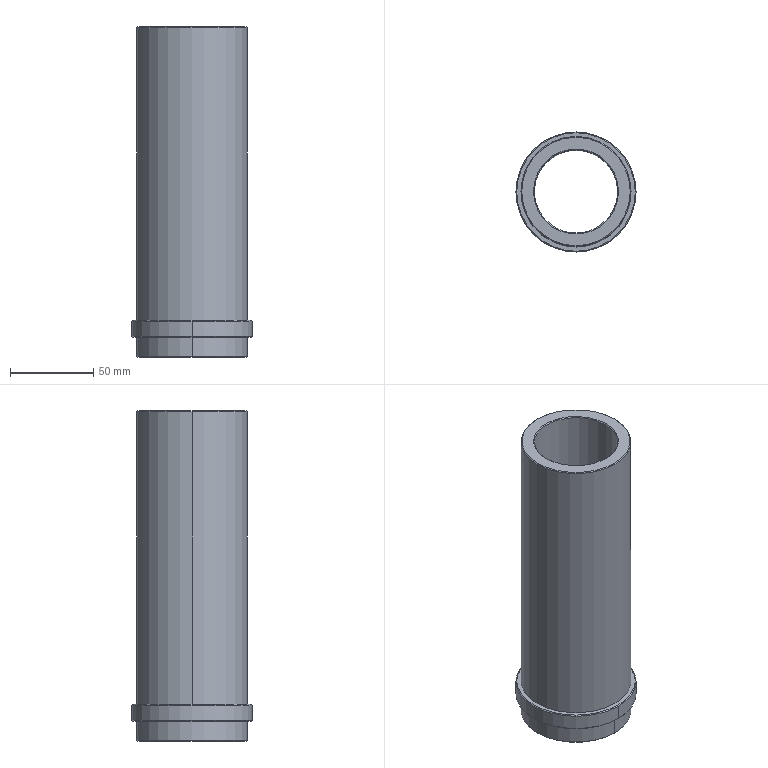Part | Creo | 1 solid | 24 faces | box 72 x 72 x 198 mm | volume 294980 mm3 | cone 12 | cylinder 8 | plane 4 | commonest cylinder face diameters 66 x4 50 x2 72 x2
STEP:
#1=CARTESIAN_POINT('',(230.,291.995,-15.5));
#2=VERTEX_POINT('',#1);
#3=CARTESIAN_POINT('',(280.,291.995,-15.5));
#4=VERTEX_POINT('',#3);
#5=CARTESIAN_POINT('',(255.,291.995,-15.5));
#6=DIRECTION('',(0.,0.,-1.));
#7=DIRECTION('',(-1.,0.,0.));
#8=AXIS2_PLACEMENT_3D('',#5,#6,#7);
#9=CIRCLE('',#8,25.);
#10=EDGE_CURVE('',#2,#4,#9,.T.);
#11=ORIENTED_EDGE('',*,*,#10,.T.);
#12=CARTESIAN_POINT('',(280.,291.995,-212.5));
#13=VERTEX_POINT('',#12);
#14=CARTESIAN_POINT('',(280.,291.995,-212.5));
#15=DIRECTION('',(0.,0.,1.));
#16=VECTOR('',#15,197.);
#17=LINE('',#14,#16);
#18=EDGE_CURVE('',#13,#4,#17,.T.);
#19=ORIENTED_EDGE('',*,*,#18,.F.);
#20=CARTESIAN_POINT('',(230.,291.995,-212.5));
#21=VERTEX_POINT('',#20);
#22=CARTESIAN_POINT('',(255.,291.995,-212.5));
#23=DIRECTION('',(0.,0.,1.));
#24=DIRECTION('',(1.,0.,0.));
#25=AXIS2_PLACEMENT_3D('',#22,#23,#24);
#26=CIRCLE('',#25,25.);
#27=EDGE_CURVE('',#13,#21,#26,.T.);
#28=ORIENTED_EDGE('',*,*,#27,.T.);
#29=CARTESIAN_POINT('',(230.,291.995,-212.5));
#30=DIRECTION('',(0.,0.,1.));
#31=VECTOR('',#30,197.);
#32=LINE('',#29,#31);
#33=EDGE_CURVE('',#21,#2,#32,.T.);
#34=ORIENTED_EDGE('',*,*,#33,.T.);
#35=EDGE_LOOP('',(#11,#19,#28,#34));
#36=FACE_OUTER_BOUND('',#35,.F.);
#37=CARTESIAN_POINT('',(255.,291.995,-201.));
#38=DIRECTION('',(0.,0.,1.));
#39=DIRECTION('',(1.,0.,0.));
#40=AXIS2_PLACEMENT_3D('',#37,#38,#39);
#41=CYLINDRICAL_SURFACE('',#40,25.);
#42=ADVANCED_FACE('',(#36),#41,.F.);
#43=CARTESIAN_POINT('',(229.5,291.995,-15.));
#44=VERTEX_POINT('',#43);
#45=CARTESIAN_POINT('',(280.5,291.995,-15.));
#46=VERTEX_POINT('',#45);
#47=CARTESIAN_POINT('',(255.,291.995,-15.));
#48=DIRECTION('',(0.,0.,-1.));
#49=DIRECTION('',(-1.,0.,0.));
#50=AXIS2_PLACEMENT_3D('',#47,#48,#49);
#51=CIRCLE('',#50,25.5);
#52=EDGE_CURVE('',#44,#46,#51,.T.);
#53=ORIENTED_EDGE('',*,*,#52,.T.);
#54=CARTESIAN_POINT('',(280.,291.995,-15.5));
#55=DIRECTION('',(0.7071,0.,0.7071));
#56=VECTOR('',#55,0.7071);
#57=LINE('',#54,#56);
#58=EDGE_CURVE('',#4,#46,#57,.T.);
#59=ORIENTED_EDGE('',*,*,#58,.F.);
#60=ORIENTED_EDGE('',*,*,#10,.F.);
#61=CARTESIAN_POINT('',(230.,291.995,-15.5));
#62=DIRECTION('',(-0.7071,0.,0.7071));
#63=VECTOR('',#62,0.7071);
#64=LINE('',#61,#63);
#65=EDGE_CURVE('',#2,#44,#64,.T.);
#66=ORIENTED_EDGE('',*,*,#65,.T.);
#67=EDGE_LOOP('',(#53,#59,#60,#66));
#68=FACE_OUTER_BOUND('',#67,.F.);
#69=CARTESIAN_POINT('',(255.,291.995,-15.25));
#70=DIRECTION('',(0.,0.,1.));
#71=DIRECTION('',(-1.,0.,0.));
#72=AXIS2_PLACEMENT_3D('',#69,#70,#71);
#73=CONICAL_SURFACE('',#72,25.25,45.);
#74=ADVANCED_FACE('',(#68),#73,.F.);
#75=CARTESIAN_POINT('',(287.5,291.995,-15.));
#76=VERTEX_POINT('',#75);
#77=CARTESIAN_POINT('',(222.5,291.995,-15.));
#78=VERTEX_POINT('',#77);
#79=CARTESIAN_POINT('',(255.,291.995,-15.));
#80=DIRECTION('',(0.,0.,1.));
#81=DIRECTION('',(1.,0.,0.));
#82=AXIS2_PLACEMENT_3D('',#79,#80,#81);
#83=CIRCLE('',#82,32.5);
#84=EDGE_CURVE('',#76,#78,#83,.T.);
#85=ORIENTED_EDGE('',*,*,#84,.F.);
#86=CARTESIAN_POINT('',(255.,291.995,-15.));
#87=DIRECTION('',(0.,0.,1.));
#88=DIRECTION('',(-1.,0.,0.));
#89=AXIS2_PLACEMENT_3D('',#86,#87,#88);
#90=CIRCLE('',#89,32.5);
#91=EDGE_CURVE('',#78,#76,#90,.T.);
#92=ORIENTED_EDGE('',*,*,#91,.F.);
#93=EDGE_LOOP('',(#85,#92));
#94=FACE_OUTER_BOUND('',#93,.F.);
#95=CARTESIAN_POINT('',(255.,291.995,-15.));
#96=DIRECTION('',(0.,0.,-1.));
#97=DIRECTION('',(1.,0.,0.));
#98=AXIS2_PLACEMENT_3D('',#95,#96,#97);
#99=CIRCLE('',#98,25.5);
#100=EDGE_CURVE('',#46,#44,#99,.T.);
#101=ORIENTED_EDGE('',*,*,#100,.F.);
#102=ORIENTED_EDGE('',*,*,#52,.F.);
#103=EDGE_LOOP('',(#101,#102));
#104=FACE_BOUND('',#103,.F.);
#105=CARTESIAN_POINT('',(-210.,43.995,-15.));
#106=DIRECTION('',(0.,0.,1.));
#107=DIRECTION('',(1.,0.,0.));
#108=AXIS2_PLACEMENT_3D('',#105,#106,#107);
#109=PLANE('',#108);
#110=ADVANCED_FACE('',(#94,#104),#109,.T.);
#111=ORIENTED_EDGE('',*,*,#100,.T.);
#112=ORIENTED_EDGE('',*,*,#65,.F.);
#113=CARTESIAN_POINT('',(255.,291.995,-15.5));
#114=DIRECTION('',(0.,0.,-1.));
#115=DIRECTION('',(1.,0.,0.));
#116=AXIS2_PLACEMENT_3D('',#113,#114,#115);
#117=CIRCLE('',#116,25.);
#118=EDGE_CURVE('',#4,#2,#117,.T.);
#119=ORIENTED_EDGE('',*,*,#118,.F.);
#120=ORIENTED_EDGE('',*,*,#58,.T.);
#121=EDGE_LOOP('',(#111,#112,#119,#120));
#122=FACE_OUTER_BOUND('',#121,.F.);
#123=CARTESIAN_POINT('',(255.,291.995,-15.25));
#124=DIRECTION('',(0.,0.,1.));
#125=DIRECTION('',(-1.,0.,0.));
#126=AXIS2_PLACEMENT_3D('',#123,#124,#125);
#127=CONICAL_SURFACE('',#126,25.25,45.);
#128=ADVANCED_FACE('',(#122),#127,.F.);
#129=ORIENTED_EDGE('',*,*,#118,.T.);
#130=ORIENTED_EDGE('',*,*,#33,.F.);
#131=CARTESIAN_POINT('',(255.,266.995,-212.5));
#132=VERTEX_POINT('',#131);
#133=CARTESIAN_POINT('',(255.,291.995,-212.5));
#134=DIRECTION('',(0.,0.,1.));
#135=DIRECTION('',(-1.,0.,0.));
#136=AXIS2_PLACEMENT_3D('',#133,#134,#135);
#137=CIRCLE('',#136,25.);
#138=EDGE_CURVE('',#21,#132,#137,.T.);
#139=ORIENTED_EDGE('',*,*,#138,.T.);
#140=CARTESIAN_POINT('',(255.,291.995,-212.5));
#141=DIRECTION('',(0.,0.,1.));
#142=DIRECTION('',(0.,-1.,0.));
#143=AXIS2_PLACEMENT_3D('',#140,#141,#142);
#144=CIRCLE('',#143,25.);
#145=EDGE_CURVE('',#132,#13,#144,.T.);
#146=ORIENTED_EDGE('',*,*,#145,.T.);
#147=ORIENTED_EDGE('',*,*,#18,.T.);
#148=EDGE_LOOP('',(#129,#130,#139,#146,#147));
#149=FACE_OUTER_BOUND('',#148,.F.);
#150=CARTESIAN_POINT('',(255.,291.995,-201.));
#151=DIRECTION('',(0.,0.,1.));
#152=DIRECTION('',(1.,0.,0.));
#153=AXIS2_PLACEMENT_3D('',#150,#151,#152);
#154=CYLINDRICAL_SURFACE('',#153,25.);
#155=ADVANCED_FACE('',(#149),#154,.F.);
#156=ORIENTED_EDGE('',*,*,#145,.F.);
#157=ORIENTED_EDGE('',*,*,#138,.F.);
#158=CARTESIAN_POINT('',(229.5,291.995,-213.));
#159=VERTEX_POINT('',#158);
#160=CARTESIAN_POINT('',(230.,291.995,-212.5));
#161=DIRECTION('',(-0.7071,0.,-0.7071));
#162=VECTOR('',#161,0.7071);
#163=LINE('',#160,#162);
#164=EDGE_CURVE('',#21,#159,#163,.T.);
#165=ORIENTED_EDGE('',*,*,#164,.T.);
#166=CARTESIAN_POINT('',(255.,266.495,-213.));
#167=VERTEX_POINT('',#166);
#168=CARTESIAN_POINT('',(255.,291.995,-213.));
#169=DIRECTION('',(0.,0.,1.));
#170=DIRECTION('',(-1.,0.,0.));
#171=AXIS2_PLACEMENT_3D('',#168,#169,#170);
#172=CIRCLE('',#171,25.5);
#173=EDGE_CURVE('',#159,#167,#172,.T.);
#174=ORIENTED_EDGE('',*,*,#173,.T.);
#175=CARTESIAN_POINT('',(280.5,291.995,-213.));
#176=VERTEX_POINT('',#175);
#177=CARTESIAN_POINT('',(255.,291.995,-213.));
#178=DIRECTION('',(0.,0.,1.));
#179=DIRECTION('',(0.,-1.,0.));
#180=AXIS2_PLACEMENT_3D('',#177,#178,#179);
#181=CIRCLE('',#180,25.5);
#182=EDGE_CURVE('',#167,#176,#181,.T.);
#183=ORIENTED_EDGE('',*,*,#182,.T.);
#184=CARTESIAN_POINT('',(280.,291.995,-212.5));
#185=DIRECTION('',(0.7071,0.,-0.7071));
#186=VECTOR('',#185,0.7071);
#187=LINE('',#184,#186);
#188=EDGE_CURVE('',#13,#176,#187,.T.);
#189=ORIENTED_EDGE('',*,*,#188,.F.);
#190=EDGE_LOOP('',(#156,#157,#165,#174,#183,#189));
#191=FACE_OUTER_BOUND('',#190,.F.);
#192=CARTESIAN_POINT('',(255.,291.995,-212.75));
#193=DIRECTION('',(0.,0.,-1.));
#194=DIRECTION('',(-1.,0.,0.));
#195=AXIS2_PLACEMENT_3D('',#192,#193,#194);
#196=CONICAL_SURFACE('',#195,25.25,45.);
#197=ADVANCED_FACE('',(#191),#196,.F.);
#198=ORIENTED_EDGE('',*,*,#27,.F.);
#199=ORIENTED_EDGE('',*,*,#188,.T.);
#200=CARTESIAN_POINT('',(255.,317.495,-213.));
#201=VERTEX_POINT('',#200);
#202=CARTESIAN_POINT('',(255.,291.995,-213.));
#203=DIRECTION('',(0.,0.,1.));
#204=DIRECTION('',(1.,0.,0.));
#205=AXIS2_PLACEMENT_3D('',#202,#203,#204);
#206=CIRCLE('',#205,25.5);
#207=EDGE_CURVE('',#176,#201,#206,.T.);
#208=ORIENTED_EDGE('',*,*,#207,.T.);
#209=CARTESIAN_POINT('',(255.,291.995,-213.));
#210=DIRECTION('',(0.,0.,1.));
#211=DIRECTION('',(0.,1.,0.));
#212=AXIS2_PLACEMENT_3D('',#209,#210,#211);
#213=CIRCLE('',#212,25.5);
#214=EDGE_CURVE('',#201,#159,#213,.T.);
#215=ORIENTED_EDGE('',*,*,#214,.T.);
#216=ORIENTED_EDGE('',*,*,#164,.F.);
#217=EDGE_LOOP('',(#198,#199,#208,#215,#216));
#218=FACE_OUTER_BOUND('',#217,.F.);
#219=CARTESIAN_POINT('',(255.,291.995,-212.75));
#220=DIRECTION('',(0.,0.,-1.));
#221=DIRECTION('',(-1.,0.,0.));
#222=AXIS2_PLACEMENT_3D('',#219,#220,#221);
#223=CONICAL_SURFACE('',#222,25.25,45.);
#224=ADVANCED_FACE('',(#218),#223,.F.);
#225=CARTESIAN_POINT('',(255.,324.495,-213.));
#226=VERTEX_POINT('',#225);
#227=CARTESIAN_POINT('',(287.5,291.995,-213.));
#228=VERTEX_POINT('',#227);
#229=CARTESIAN_POINT('',(255.,291.995,-213.));
#230=DIRECTION('',(0.,0.,-1.));
#231=DIRECTION('',(0.,1.,0.));
#232=AXIS2_PLACEMENT_3D('',#229,#230,#231);
#233=CIRCLE('',#232,32.5);
#234=EDGE_CURVE('',#226,#228,#233,.T.);
#235=ORIENTED_EDGE('',*,*,#234,.F.);
#236=CARTESIAN_POINT('',(222.5,291.995,-213.));
#237=VERTEX_POINT('',#236);
#238=CARTESIAN_POINT('',(255.,291.995,-213.));
#239=DIRECTION('',(0.,0.,-1.));
#240=DIRECTION('',(-1.,0.,0.));
#241=AXIS2_PLACEMENT_3D('',#238,#239,#240);
#242=CIRCLE('',#241,32.5);
#243=EDGE_CURVE('',#237,#226,#242,.T.);
#244=ORIENTED_EDGE('',*,*,#243,.F.);
#245=CARTESIAN_POINT('',(255.,259.495,-213.));
#246=VERTEX_POINT('',#245);
#247=CARTESIAN_POINT('',(255.,291.995,-213.));
#248=DIRECTION('',(0.,0.,-1.));
#249=DIRECTION('',(0.,-1.,0.));
#250=AXIS2_PLACEMENT_3D('',#247,#248,#249);
#251=CIRCLE('',#250,32.5);
#252=EDGE_CURVE('',#246,#237,#251,.T.);
#253=ORIENTED_EDGE('',*,*,#252,.F.);
#254=CARTESIAN_POINT('',(255.,291.995,-213.));
#255=DIRECTION('',(0.,0.,-1.));
#256=DIRECTION('',(1.,0.,0.));
#257=AXIS2_PLACEMENT_3D('',#254,#255,#256);
#258=CIRCLE('',#257,32.5);
#259=EDGE_CURVE('',#228,#246,#258,.T.);
#260=ORIENTED_EDGE('',*,*,#259,.F.);
#261=EDGE_LOOP('',(#235,#244,#253,#260));
#262=FACE_OUTER_BOUND('',#261,.F.);
#263=ORIENTED_EDGE('',*,*,#182,.F.);
#264=ORIENTED_EDGE('',*,*,#173,.F.);
#265=ORIENTED_EDGE('',*,*,#214,.F.);
#266=ORIENTED_EDGE('',*,*,#207,.F.);
#267=EDGE_LOOP('',(#263,#264,#265,#266));
#268=FACE_BOUND('',#267,.F.);
#269=CARTESIAN_POINT('',(65.,43.995,-213.));
#270=DIRECTION('',(0.,0.,-1.));
#271=DIRECTION('',(0.,1.,0.));
#272=AXIS2_PLACEMENT_3D('',#269,#270,#271);
#273=PLANE('',#272);
#274=ADVANCED_FACE('',(#262,#268),#273,.T.);
#275=CARTESIAN_POINT('',(255.,324.995,-212.5));
#276=VERTEX_POINT('',#275);
#277=CARTESIAN_POINT('',(288.,291.995,-212.5));
#278=VERTEX_POINT('',#277);
#279=CARTESIAN_POINT('',(255.,291.995,-212.5));
#280=DIRECTION('',(0.,0.,-1.));
#281=DIRECTION('',(0.,1.,0.));
#282=AXIS2_PLACEMENT_3D('',#279,#280,#281);
#283=CIRCLE('',#282,33.);
#284=EDGE_CURVE('',#276,#278,#283,.T.);
#285=ORIENTED_EDGE('',*,*,#284,.F.);
#286=CARTESIAN_POINT('',(222.,291.995,-212.5));
#287=VERTEX_POINT('',#286);
#288=CARTESIAN_POINT('',(255.,291.995,-212.5));
#289=DIRECTION('',(0.,0.,-1.));
#290=DIRECTION('',(-1.,0.,0.));
#291=AXIS2_PLACEMENT_3D('',#288,#289,#290);
#292=CIRCLE('',#291,33.);
#293=EDGE_CURVE('',#287,#276,#292,.T.);
#294=ORIENTED_EDGE('',*,*,#293,.F.);
#295=CARTESIAN_POINT('',(222.5,291.995,-213.));
#296=DIRECTION('',(-0.7071,0.,0.7071));
#297=VECTOR('',#296,0.7071);
#298=LINE('',#295,#297);
#299=EDGE_CURVE('',#237,#287,#298,.T.);
#300=ORIENTED_EDGE('',*,*,#299,.F.);
#301=ORIENTED_EDGE('',*,*,#243,.T.);
#302=ORIENTED_EDGE('',*,*,#234,.T.);
#303=CARTESIAN_POINT('',(287.5,291.995,-213.));
#304=DIRECTION('',(0.7071,0.,0.7071));
#305=VECTOR('',#304,0.7071);
#306=LINE('',#303,#305);
#307=EDGE_CURVE('',#228,#278,#306,.T.);
#308=ORIENTED_EDGE('',*,*,#307,.T.);
#309=EDGE_LOOP('',(#285,#294,#300,#301,#302,#308));
#310=FACE_OUTER_BOUND('',#309,.F.);
#311=CARTESIAN_POINT('',(255.,291.995,-212.75));
#312=DIRECTION('',(0.,0.,1.));
#313=DIRECTION('',(-1.,0.,0.));
#314=AXIS2_PLACEMENT_3D('',#311,#312,#313);
#315=CONICAL_SURFACE('',#314,32.75,45.);
#316=ADVANCED_FACE('',(#310),#315,.T.);
#317=CARTESIAN_POINT('',(255.,258.995,-212.5));
#318=VERTEX_POINT('',#317);
#319=CARTESIAN_POINT('',(255.,291.995,-212.5));
#320=DIRECTION('',(0.,0.,-1.));
#321=DIRECTION('',(1.,0.,0.));
#322=AXIS2_PLACEMENT_3D('',#319,#320,#321);
#323=CIRCLE('',#322,33.);
#324=EDGE_CURVE('',#278,#318,#323,.T.);
#325=ORIENTED_EDGE('',*,*,#324,.T.);
#326=CARTESIAN_POINT('',(255.,258.995,-201.));
#327=VERTEX_POINT('',#326);
#328=CARTESIAN_POINT('',(255.,258.995,-201.));
#329=DIRECTION('',(0.,0.,-1.));
#330=VECTOR('',#329,11.5);
#331=LINE('',#328,#330);
#332=EDGE_CURVE('',#327,#318,#331,.T.);
#333=ORIENTED_EDGE('',*,*,#332,.F.);
#334=CARTESIAN_POINT('',(255.,324.995,-201.));
#335=VERTEX_POINT('',#334);
#336=CARTESIAN_POINT('',(255.,291.995,-201.));
#337=DIRECTION('',(0.,0.,1.));
#338=DIRECTION('',(0.,-1.,0.));
#339=AXIS2_PLACEMENT_3D('',#336,#337,#338);
#340=CIRCLE('',#339,33.);
#341=EDGE_CURVE('',#327,#335,#340,.T.);
#342=ORIENTED_EDGE('',*,*,#341,.T.);
#343=CARTESIAN_POINT('',(255.,324.995,-201.));
#344=DIRECTION('',(0.,0.,-1.));
#345=VECTOR('',#344,11.5);
#346=LINE('',#343,#345);
#347=EDGE_CURVE('',#335,#276,#346,.T.);
#348=ORIENTED_EDGE('',*,*,#347,.T.);
#349=ORIENTED_EDGE('',*,*,#284,.T.);
#350=EDGE_LOOP('',(#325,#333,#342,#348,#349));
#351=FACE_OUTER_BOUND('',#350,.F.);
#352=CARTESIAN_POINT('',(255.,291.995,-201.));
#353=DIRECTION('',(0.,0.,-1.));
#354=DIRECTION('',(0.,1.,0.));
#355=AXIS2_PLACEMENT_3D('',#352,#353,#354);
#356=CYLINDRICAL_SURFACE('',#355,33.);
#357=ADVANCED_FACE('',(#351),#356,.T.);
#358=ORIENTED_EDGE('',*,*,#324,.F.);
#359=ORIENTED_EDGE('',*,*,#307,.F.);
#360=ORIENTED_EDGE('',*,*,#259,.T.);
#361=ORIENTED_EDGE('',*,*,#252,.T.);
#362=ORIENTED_EDGE('',*,*,#299,.T.);
#363=CARTESIAN_POINT('',(255.,291.995,-212.5));
#364=DIRECTION('',(0.,0.,-1.));
#365=DIRECTION('',(0.,-1.,0.));
#366=AXIS2_PLACEMENT_3D('',#363,#364,#365);
#367=CIRCLE('',#366,33.);
#368=EDGE_CURVE('',#318,#287,#367,.T.);
#369=ORIENTED_EDGE('',*,*,#368,.F.);
#370=EDGE_LOOP('',(#358,#359,#360,#361,#362,#369));
#371=FACE_OUTER_BOUND('',#370,.F.);
#372=CARTESIAN_POINT('',(255.,291.995,-212.75));
#373=DIRECTION('',(0.,0.,1.));
#374=DIRECTION('',(-1.,0.,0.));
#375=AXIS2_PLACEMENT_3D('',#372,#373,#374);
#376=CONICAL_SURFACE('',#375,32.75,45.);
#377=ADVANCED_FACE('',(#371),#376,.T.);
#378=ORIENTED_EDGE('',*,*,#293,.T.);
#379=ORIENTED_EDGE('',*,*,#347,.F.);
#380=CARTESIAN_POINT('',(255.,291.995,-201.));
#381=DIRECTION('',(0.,0.,1.));
#382=DIRECTION('',(0.,1.,0.));
#383=AXIS2_PLACEMENT_3D('',#380,#381,#382);
#384=CIRCLE('',#383,33.);
#385=EDGE_CURVE('',#335,#327,#384,.T.);
#386=ORIENTED_EDGE('',*,*,#385,.T.);
#387=ORIENTED_EDGE('',*,*,#332,.T.);
#388=ORIENTED_EDGE('',*,*,#368,.T.);
#389=EDGE_LOOP('',(#378,#379,#386,#387,#388));
#390=FACE_OUTER_BOUND('',#389,.F.);
#391=CARTESIAN_POINT('',(255.,291.995,-201.));
#392=DIRECTION('',(0.,0.,-1.));
#393=DIRECTION('',(0.,1.,0.));
#394=AXIS2_PLACEMENT_3D('',#391,#392,#393);
#395=CYLINDRICAL_SURFACE('',#394,33.);
#396=ADVANCED_FACE('',(#390),#395,.T.);
#397=CARTESIAN_POINT('',(255.,327.495,-201.));
#398=VERTEX_POINT('',#397);
#399=CARTESIAN_POINT('',(290.5,291.995,-201.));
#400=VERTEX_POINT('',#399);
#401=CARTESIAN_POINT('',(255.,291.995,-201.));
#402=DIRECTION('',(0.,0.,-1.));
#403=DIRECTION('',(0.,1.,0.));
#404=AXIS2_PLACEMENT_3D('',#401,#402,#403);
#405=CIRCLE('',#404,35.5);
#406=EDGE_CURVE('',#398,#400,#405,.T.);
#407=ORIENTED_EDGE('',*,*,#406,.F.);
#408=CARTESIAN_POINT('',(219.5,291.995,-201.));
#409=VERTEX_POINT('',#408);
#410=CARTESIAN_POINT('',(255.,291.995,-201.));
#411=DIRECTION('',(0.,0.,-1.));
#412=DIRECTION('',(-1.,0.,0.));
#413=AXIS2_PLACEMENT_3D('',#410,#411,#412);
#414=CIRCLE('',#413,35.5);
#415=EDGE_CURVE('',#409,#398,#414,.T.);
#416=ORIENTED_EDGE('',*,*,#415,.F.);
#417=CARTESIAN_POINT('',(255.,256.495,-201.));
#418=VERTEX_POINT('',#417);
#419=CARTESIAN_POINT('',(255.,291.995,-201.));
#420=DIRECTION('',(0.,0.,-1.));
#421=DIRECTION('',(0.,-1.,0.));
#422=AXIS2_PLACEMENT_3D('',#419,#420,#421);
#423=CIRCLE('',#422,35.5);
#424=EDGE_CURVE('',#418,#409,#423,.T.);
#425=ORIENTED_EDGE('',*,*,#424,.F.);
#426=CARTESIAN_POINT('',(255.,291.995,-201.));
#427=DIRECTION('',(0.,0.,-1.));
#428=DIRECTION('',(1.,0.,0.));
#429=AXIS2_PLACEMENT_3D('',#426,#427,#428);
#430=CIRCLE('',#429,35.5);
#431=EDGE_CURVE('',#400,#418,#430,.T.);
#432=ORIENTED_EDGE('',*,*,#431,.F.);
#433=EDGE_LOOP('',(#407,#416,#425,#432));
#434=FACE_OUTER_BOUND('',#433,.F.);
#435=ORIENTED_EDGE('',*,*,#385,.F.);
#436=ORIENTED_EDGE('',*,*,#341,.F.);
#437=EDGE_LOOP('',(#435,#436));
#438=FACE_BOUND('',#437,.F.);
#439=CARTESIAN_POINT('',(-210.,43.995,-201.));
#440=DIRECTION('',(0.,0.,1.));
#441=DIRECTION('',(1.,0.,0.));
#442=AXIS2_PLACEMENT_3D('',#439,#440,#441);
#443=PLANE('',#442);
#444=ADVANCED_FACE('',(#434,#438),#443,.F.);
#445=CARTESIAN_POINT('',(219.,291.995,-200.5));
#446=VERTEX_POINT('',#445);
#447=CARTESIAN_POINT('',(255.,327.995,-200.5));
#448=VERTEX_POINT('',#447);
#449=CARTESIAN_POINT('',(255.,291.995,-200.5));
#450=DIRECTION('',(0.,0.,-1.));
#451=DIRECTION('',(-1.,0.,0.));
#452=AXIS2_PLACEMENT_3D('',#449,#450,#451);
#453=CIRCLE('',#452,36.);
#454=EDGE_CURVE('',#446,#448,#453,.T.);
#455=ORIENTED_EDGE('',*,*,#454,.F.);
#456=CARTESIAN_POINT('',(219.5,291.995,-201.));
#457=DIRECTION('',(-0.7071,0.,0.7071));
#458=VECTOR('',#457,0.7071);
#459=LINE('',#456,#458);
#460=EDGE_CURVE('',#409,#446,#459,.T.);
#461=ORIENTED_EDGE('',*,*,#460,.F.);
#462=ORIENTED_EDGE('',*,*,#415,.T.);
#463=ORIENTED_EDGE('',*,*,#406,.T.);
#464=CARTESIAN_POINT('',(291.,291.995,-200.5));
#465=VERTEX_POINT('',#464);
#466=CARTESIAN_POINT('',(290.5,291.995,-201.));
#467=DIRECTION('',(0.7071,0.,0.7071));
#468=VECTOR('',#467,0.7071);
#469=LINE('',#466,#468);
#470=EDGE_CURVE('',#400,#465,#469,.T.);
#471=ORIENTED_EDGE('',*,*,#470,.T.);
#472=CARTESIAN_POINT('',(255.,291.995,-200.5));
#473=DIRECTION('',(0.,0.,-1.));
#474=DIRECTION('',(0.,1.,0.));
#475=AXIS2_PLACEMENT_3D('',#472,#473,#474);
#476=CIRCLE('',#475,36.);
#477=EDGE_CURVE('',#448,#465,#476,.T.);
#478=ORIENTED_EDGE('',*,*,#477,.F.);
#479=EDGE_LOOP('',(#455,#461,#462,#463,#471,#478));
#480=FACE_OUTER_BOUND('',#479,.F.);
#481=CARTESIAN_POINT('',(255.,291.995,-200.75));
#482=DIRECTION('',(0.,0.,1.));
#483=DIRECTION('',(-1.,0.,0.));
#484=AXIS2_PLACEMENT_3D('',#481,#482,#483);
#485=CONICAL_SURFACE('',#484,35.75,45.);
#486=ADVANCED_FACE('',(#480),#485,.T.);
#487=CARTESIAN_POINT('',(219.,291.995,-191.5));
#488=VERTEX_POINT('',#487);
#489=CARTESIAN_POINT('',(255.,255.995,-191.5));
#490=VERTEX_POINT('',#489);
#491=CARTESIAN_POINT('',(255.,291.995,-191.5));
#492=DIRECTION('',(0.,0.,1.));
#493=DIRECTION('',(-1.,0.,0.));
#494=AXIS2_PLACEMENT_3D('',#491,#492,#493);
#495=CIRCLE('',#494,36.);
#496=EDGE_CURVE('',#488,#490,#495,.T.);
#497=ORIENTED_EDGE('',*,*,#496,.T.);
#498=CARTESIAN_POINT('',(255.,255.995,-200.5));
#499=VERTEX_POINT('',#498);
#500=CARTESIAN_POINT('',(255.,255.995,-191.5));
#501=DIRECTION('',(0.,0.,-1.));
#502=VECTOR('',#501,9.);
#503=LINE('',#500,#502);
#504=EDGE_CURVE('',#490,#499,#503,.T.);
#505=ORIENTED_EDGE('',*,*,#504,.T.);
#506=CARTESIAN_POINT('',(255.,291.995,-200.5));
#507=DIRECTION('',(0.,0.,-1.));
#508=DIRECTION('',(0.,-1.,0.));
#509=AXIS2_PLACEMENT_3D('',#506,#507,#508);
#510=CIRCLE('',#509,36.);
#511=EDGE_CURVE('',#499,#446,#510,.T.);
#512=ORIENTED_EDGE('',*,*,#511,.T.);
#513=ORIENTED_EDGE('',*,*,#454,.T.);
#514=CARTESIAN_POINT('',(255.,327.995,-191.5));
#515=VERTEX_POINT('',#514);
#516=CARTESIAN_POINT('',(255.,327.995,-191.5));
#517=DIRECTION('',(0.,0.,-1.));
#518=VECTOR('',#517,9.);
#519=LINE('',#516,#518);
#520=EDGE_CURVE('',#515,#448,#519,.T.);
#521=ORIENTED_EDGE('',*,*,#520,.F.);
#522=CARTESIAN_POINT('',(255.,291.995,-191.5));
#523=DIRECTION('',(0.,0.,1.));
#524=DIRECTION('',(0.,1.,0.));
#525=AXIS2_PLACEMENT_3D('',#522,#523,#524);
#526=CIRCLE('',#525,36.);
#527=EDGE_CURVE('',#515,#488,#526,.T.);
#528=ORIENTED_EDGE('',*,*,#527,.T.);
#529=EDGE_LOOP('',(#497,#505,#512,#513,#521,#528));
#530=FACE_OUTER_BOUND('',#529,.F.);
#531=CARTESIAN_POINT('',(255.,291.995,-201.));
#532=DIRECTION('',(0.,0.,-1.));
#533=DIRECTION('',(0.,1.,0.));
#534=AXIS2_PLACEMENT_3D('',#531,#532,#533);
#535=CYLINDRICAL_SURFACE('',#534,36.);
#536=ADVANCED_FACE('',(#530),#535,.T.);
#537=CARTESIAN_POINT('',(291.,291.995,-191.5));
#538=VERTEX_POINT('',#537);
#539=CARTESIAN_POINT('',(255.,291.995,-191.5));
#540=DIRECTION('',(0.,0.,1.));
#541=DIRECTION('',(0.,-1.,0.));
#542=AXIS2_PLACEMENT_3D('',#539,#540,#541);
#543=CIRCLE('',#542,36.);
#544=EDGE_CURVE('',#490,#538,#543,.T.);
#545=ORIENTED_EDGE('',*,*,#544,.F.);
#546=ORIENTED_EDGE('',*,*,#496,.F.);
#547=CARTESIAN_POINT('',(219.5,291.995,-191.));
#548=VERTEX_POINT('',#547);
#549=CARTESIAN_POINT('',(219.5,291.995,-191.));
#550=DIRECTION('',(-0.7071,0.,-0.7071));
#551=VECTOR('',#550,0.7071);
#552=LINE('',#549,#551);
#553=EDGE_CURVE('',#548,#488,#552,.T.);
#554=ORIENTED_EDGE('',*,*,#553,.F.);
#555=CARTESIAN_POINT('',(255.,256.495,-191.));
#556=VERTEX_POINT('',#555);
#557=CARTESIAN_POINT('',(255.,291.995,-191.));
#558=DIRECTION('',(0.,0.,1.));
#559=DIRECTION('',(-1.,0.,0.));
#560=AXIS2_PLACEMENT_3D('',#557,#558,#559);
#561=CIRCLE('',#560,35.5);
#562=EDGE_CURVE('',#548,#556,#561,.T.);
#563=ORIENTED_EDGE('',*,*,#562,.T.);
#564=CARTESIAN_POINT('',(290.5,291.995,-191.));
#565=VERTEX_POINT('',#564);
#566=CARTESIAN_POINT('',(255.,291.995,-191.));
#567=DIRECTION('',(0.,0.,1.));
#568=DIRECTION('',(0.,-1.,0.));
#569=AXIS2_PLACEMENT_3D('',#566,#567,#568);
#570=CIRCLE('',#569,35.5);
#571=EDGE_CURVE('',#556,#565,#570,.T.);
#572=ORIENTED_EDGE('',*,*,#571,.T.);
#573=CARTESIAN_POINT('',(290.5,291.995,-191.));
#574=DIRECTION('',(0.7071,0.,-0.7071));
#575=VECTOR('',#574,0.7071);
#576=LINE('',#573,#575);
#577=EDGE_CURVE('',#565,#538,#576,.T.);
#578=ORIENTED_EDGE('',*,*,#577,.T.);
#579=EDGE_LOOP('',(#545,#546,#554,#563,#572,#578));
#580=FACE_OUTER_BOUND('',#579,.F.);
#581=CARTESIAN_POINT('',(255.,291.995,-191.25));
#582=DIRECTION('',(0.,0.,-1.));
#583=DIRECTION('',(-1.,0.,0.));
#584=AXIS2_PLACEMENT_3D('',#581,#582,#583);
#585=CONICAL_SURFACE('',#584,35.75,45.);
#586=ADVANCED_FACE('',(#580),#585,.T.);
#587=CARTESIAN_POINT('',(255.,291.995,-191.5));
#588=DIRECTION('',(0.,0.,1.));
#589=DIRECTION('',(1.,0.,0.));
#590=AXIS2_PLACEMENT_3D('',#587,#588,#589);
#591=CIRCLE('',#590,36.);
#592=EDGE_CURVE('',#538,#515,#591,.T.);
#593=ORIENTED_EDGE('',*,*,#592,.T.);
#594=ORIENTED_EDGE('',*,*,#520,.T.);
#595=ORIENTED_EDGE('',*,*,#477,.T.);
#596=CARTESIAN_POINT('',(255.,291.995,-200.5));
#597=DIRECTION('',(0.,0.,-1.));
#598=DIRECTION('',(1.,0.,0.));
#599=AXIS2_PLACEMENT_3D('',#596,#597,#598);
#600=CIRCLE('',#599,36.);
#601=EDGE_CURVE('',#465,#499,#600,.T.);
#602=ORIENTED_EDGE('',*,*,#601,.T.);
#603=ORIENTED_EDGE('',*,*,#504,.F.);
#604=ORIENTED_EDGE('',*,*,#544,.T.);
#605=EDGE_LOOP('',(#593,#594,#595,#602,#603,#604));
#606=FACE_OUTER_BOUND('',#605,.F.);
#607=CARTESIAN_POINT('',(255.,291.995,-201.));
#608=DIRECTION('',(0.,0.,-1.));
#609=DIRECTION('',(0.,1.,0.));
#610=AXIS2_PLACEMENT_3D('',#607,#608,#609);
#611=CYLINDRICAL_SURFACE('',#610,36.);
#612=ADVANCED_FACE('',(#606),#611,.T.);
#613=ORIENTED_EDGE('',*,*,#592,.F.);
#614=ORIENTED_EDGE('',*,*,#577,.F.);
#615=CARTESIAN_POINT('',(255.,327.495,-191.));
#616=VERTEX_POINT('',#615);
#617=CARTESIAN_POINT('',(255.,291.995,-191.));
#618=DIRECTION('',(0.,0.,1.));
#619=DIRECTION('',(1.,0.,0.));
#620=AXIS2_PLACEMENT_3D('',#617,#618,#619);
#621=CIRCLE('',#620,35.5);
#622=EDGE_CURVE('',#565,#616,#621,.T.);
#623=ORIENTED_EDGE('',*,*,#622,.T.);
#624=CARTESIAN_POINT('',(255.,291.995,-191.));
#625=DIRECTION('',(0.,0.,1.));
#626=DIRECTION('',(0.,1.,0.));
#627=AXIS2_PLACEMENT_3D('',#624,#625,#626);
#628=CIRCLE('',#627,35.5);
#629=EDGE_CURVE('',#616,#548,#628,.T.);
#630=ORIENTED_EDGE('',*,*,#629,.T.);
#631=ORIENTED_EDGE('',*,*,#553,.T.);
#632=ORIENTED_EDGE('',*,*,#527,.F.);
#633=EDGE_LOOP('',(#613,#614,#623,#630,#631,#632));
#634=FACE_OUTER_BOUND('',#633,.F.);
#635=CARTESIAN_POINT('',(255.,291.995,-191.25));
#636=DIRECTION('',(0.,0.,-1.));
#637=DIRECTION('',(-1.,0.,0.));
#638=AXIS2_PLACEMENT_3D('',#635,#636,#637);
#639=CONICAL_SURFACE('',#638,35.75,45.);
#640=ADVANCED_FACE('',(#634),#639,.T.);
#641=ORIENTED_EDGE('',*,*,#571,.F.);
#642=ORIENTED_EDGE('',*,*,#562,.F.);
#643=ORIENTED_EDGE('',*,*,#629,.F.);
#644=ORIENTED_EDGE('',*,*,#622,.F.);
#645=EDGE_LOOP('',(#641,#642,#643,#644));
#646=FACE_OUTER_BOUND('',#645,.F.);
#647=CARTESIAN_POINT('',(288.,291.995,-191.));
#648=VERTEX_POINT('',#647);
#649=CARTESIAN_POINT('',(222.,291.995,-191.));
#650=VERTEX_POINT('',#649);
#651=CARTESIAN_POINT('',(255.,291.995,-191.));
#652=DIRECTION('',(0.,0.,-1.));
#653=DIRECTION('',(1.,0.,0.));
#654=AXIS2_PLACEMENT_3D('',#651,#652,#653);
#655=CIRCLE('',#654,33.);
#656=EDGE_CURVE('',#648,#650,#655,.T.);
#657=ORIENTED_EDGE('',*,*,#656,.F.);
#658=CARTESIAN_POINT('',(255.,291.995,-191.));
#659=DIRECTION('',(0.,0.,-1.));
#660=DIRECTION('',(-1.,0.,0.));
#661=AXIS2_PLACEMENT_3D('',#658,#659,#660);
#662=CIRCLE('',#661,33.);
#663=EDGE_CURVE('',#650,#648,#662,.T.);
#664=ORIENTED_EDGE('',*,*,#663,.F.);
#665=EDGE_LOOP('',(#657,#664));
#666=FACE_BOUND('',#665,.F.);
#667=CARTESIAN_POINT('',(65.,43.995,-191.));
#668=DIRECTION('',(0.,0.,-1.));
#669=DIRECTION('',(0.,1.,0.));
#670=AXIS2_PLACEMENT_3D('',#667,#668,#669);
#671=PLANE('',#670);
#672=ADVANCED_FACE('',(#646,#666),#671,.F.);
#673=ORIENTED_EDGE('',*,*,#656,.T.);
#674=CARTESIAN_POINT('',(222.,291.995,-15.5));
#675=VERTEX_POINT('',#674);
#676=CARTESIAN_POINT('',(222.,291.995,-191.));
#677=DIRECTION('',(0.,0.,1.));
#678=VECTOR('',#677,175.5);
#679=LINE('',#676,#678);
#680=EDGE_CURVE('',#650,#675,#679,.T.);
#681=ORIENTED_EDGE('',*,*,#680,.T.);
#682=CARTESIAN_POINT('',(288.,291.995,-15.5));
#683=VERTEX_POINT('',#682);
#684=CARTESIAN_POINT('',(255.,291.995,-15.5));
#685=DIRECTION('',(0.,0.,1.));
#686=DIRECTION('',(-1.,0.,0.));
#687=AXIS2_PLACEMENT_3D('',#684,#685,#686);
#688=CIRCLE('',#687,33.);
#689=EDGE_CURVE('',#675,#683,#688,.T.);
#690=ORIENTED_EDGE('',*,*,#689,.T.);
#691=CARTESIAN_POINT('',(288.,291.995,-191.));
#692=DIRECTION('',(0.,0.,1.));
#693=VECTOR('',#692,175.5);
#694=LINE('',#691,#693);
#695=EDGE_CURVE('',#648,#683,#694,.T.);
#696=ORIENTED_EDGE('',*,*,#695,.F.);
#697=EDGE_LOOP('',(#673,#681,#690,#696));
#698=FACE_OUTER_BOUND('',#697,.F.);
#699=CARTESIAN_POINT('',(255.,291.995,-201.));
#700=DIRECTION('',(0.,0.,1.));
#701=DIRECTION('',(1.,0.,0.));
#702=AXIS2_PLACEMENT_3D('',#699,#700,#701);
#703=CYLINDRICAL_SURFACE('',#702,33.);
#704=ADVANCED_FACE('',(#698),#703,.T.);
#705=ORIENTED_EDGE('',*,*,#663,.T.);
#706=ORIENTED_EDGE('',*,*,#695,.T.);
#707=CARTESIAN_POINT('',(255.,291.995,-15.5));
#708=DIRECTION('',(0.,0.,1.));
#709=DIRECTION('',(1.,0.,0.));
#710=AXIS2_PLACEMENT_3D('',#707,#708,#709);
#711=CIRCLE('',#710,33.);
#712=EDGE_CURVE('',#683,#675,#711,.T.);
#713=ORIENTED_EDGE('',*,*,#712,.T.);
#714=ORIENTED_EDGE('',*,*,#680,.F.);
#715=EDGE_LOOP('',(#705,#706,#713,#714));
#716=FACE_OUTER_BOUND('',#715,.F.);
#717=CARTESIAN_POINT('',(255.,291.995,-201.));
#718=DIRECTION('',(0.,0.,1.));
#719=DIRECTION('',(1.,0.,0.));
#720=AXIS2_PLACEMENT_3D('',#717,#718,#719);
#721=CYLINDRICAL_SURFACE('',#720,33.);
#722=ADVANCED_FACE('',(#716),#721,.T.);
#723=ORIENTED_EDGE('',*,*,#84,.T.);
#724=CARTESIAN_POINT('',(222.5,291.995,-15.));
#725=DIRECTION('',(-0.7071,0.,-0.7071));
#726=VECTOR('',#725,0.7071);
#727=LINE('',#724,#726);
#728=EDGE_CURVE('',#78,#675,#727,.T.);
#729=ORIENTED_EDGE('',*,*,#728,.T.);
#730=ORIENTED_EDGE('',*,*,#712,.F.);
#731=CARTESIAN_POINT('',(287.5,291.995,-15.));
#732=DIRECTION('',(0.7071,0.,-0.7071));
#733=VECTOR('',#732,0.7071);
#734=LINE('',#731,#733);
#735=EDGE_CURVE('',#76,#683,#734,.T.);
#736=ORIENTED_EDGE('',*,*,#735,.F.);
#737=EDGE_LOOP('',(#723,#729,#730,#736));
#738=FACE_OUTER_BOUND('',#737,.F.);
#739=CARTESIAN_POINT('',(255.,291.995,-15.25));
#740=DIRECTION('',(0.,0.,-1.));
#741=DIRECTION('',(-1.,0.,0.));
#742=AXIS2_PLACEMENT_3D('',#739,#740,#741);
#743=CONICAL_SURFACE('',#742,32.75,45.);
#744=ADVANCED_FACE('',(#738),#743,.T.);
#745=ORIENTED_EDGE('',*,*,#91,.T.);
#746=ORIENTED_EDGE('',*,*,#735,.T.);
#747=ORIENTED_EDGE('',*,*,#689,.F.);
#748=ORIENTED_EDGE('',*,*,#728,.F.);
#749=EDGE_LOOP('',(#745,#746,#747,#748));
#750=FACE_OUTER_BOUND('',#749,.F.);
#751=CARTESIAN_POINT('',(255.,291.995,-15.25));
#752=DIRECTION('',(0.,0.,-1.));
#753=DIRECTION('',(-1.,0.,0.));
#754=AXIS2_PLACEMENT_3D('',#751,#752,#753);
#755=CONICAL_SURFACE('',#754,32.75,45.);
#756=ADVANCED_FACE('',(#750),#755,.T.);
#757=ORIENTED_EDGE('',*,*,#511,.F.);
#758=ORIENTED_EDGE('',*,*,#601,.F.);
#759=ORIENTED_EDGE('',*,*,#470,.F.);
#760=ORIENTED_EDGE('',*,*,#431,.T.);
#761=ORIENTED_EDGE('',*,*,#424,.T.);
#762=ORIENTED_EDGE('',*,*,#460,.T.);
#763=EDGE_LOOP('',(#757,#758,#759,#760,#761,#762));
#764=FACE_OUTER_BOUND('',#763,.F.);
#765=CARTESIAN_POINT('',(255.,291.995,-200.75));
#766=DIRECTION('',(0.,0.,1.));
#767=DIRECTION('',(-1.,0.,0.));
#768=AXIS2_PLACEMENT_3D('',#765,#766,#767);
#769=CONICAL_SURFACE('',#768,35.75,45.);
#770=ADVANCED_FACE('',(#764),#769,.T.);
#771=CLOSED_SHELL('',(#42,#74,#110,#128,#155,#197,#224,#274,#316,#357,#377,#396,#444,#486,#536,#586,#612,#640,#672,#704,#722,#744,#756,#770));
#772=MANIFOLD_SOLID_BREP('',#771);
#773=(LENGTH_UNIT()NAMED_UNIT(*)SI_UNIT(.MILLI.,.METRE.));
#774=UNCERTAINTY_MEASURE_WITH_UNIT(LENGTH_MEASURE(0.02226),#773,'','');
#775=(NAMED_UNIT(*)PLANE_ANGLE_UNIT()SI_UNIT($,.RADIAN.));
#776=PLANE_ANGLE_MEASURE_WITH_UNIT(PLANE_ANGLE_MEASURE(0.01745),#775);
#777=(CONVERSION_BASED_UNIT('DEGREE',#776)NAMED_UNIT(*)PLANE_ANGLE_UNIT());
#778=(NAMED_UNIT(*)SI_UNIT($,.STERADIAN.)SOLID_ANGLE_UNIT());
#779=(GEOMETRIC_REPRESENTATION_CONTEXT(3)GLOBAL_UNCERTAINTY_ASSIGNED_CONTEXT((#774))GLOBAL_UNIT_ASSIGNED_CONTEXT((#773,#777,#778))REPRESENTATION_CONTEXT('',''));
#780=ADVANCED_BREP_SHAPE_REPRESENTATION('',(#772),#779);